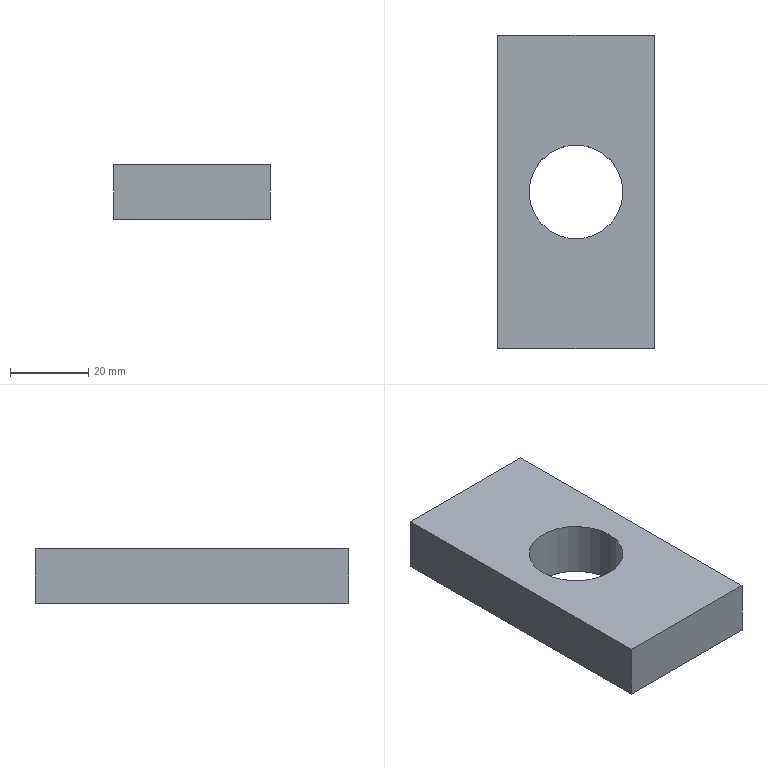Part | SolidWorks | features Extrusion 1 | 1 solid | 8 faces | box 40 x 80 x 14 mm | volume 38467 mm3 | plane 6 | cylinder 2 | commonest cylinder face diameters 24 x2
STEP:
#1=CARTESIAN_POINT('',(8.,40.,14.));
#2=VERTEX_POINT('',#1);
#3=CARTESIAN_POINT('',(32.,40.,14.));
#4=VERTEX_POINT('',#3);
#5=CARTESIAN_POINT('',(20.,40.,14.));
#6=DIRECTION('',(0.,0.,1.));
#7=DIRECTION('',(1.,0.,0.));
#8=AXIS2_PLACEMENT_3D('',#5,#6,#7);
#9=CIRCLE('',#8,12.);
#10=EDGE_CURVE('',#2,#4,#9,.T.);
#11=ORIENTED_EDGE('',*,*,#10,.T.);
#12=CARTESIAN_POINT('',(32.,40.,0.));
#13=VERTEX_POINT('',#12);
#14=CARTESIAN_POINT('',(32.,40.,14.));
#15=DIRECTION('',(0.,0.,-1.));
#16=VECTOR('',#15,1000.);
#17=LINE('',#14,#16);
#18=EDGE_CURVE('',#4,#13,#17,.T.);
#19=ORIENTED_EDGE('',*,*,#18,.T.);
#20=CARTESIAN_POINT('',(8.,40.,0.));
#21=VERTEX_POINT('',#20);
#22=CARTESIAN_POINT('',(20.,40.,0.));
#23=DIRECTION('',(0.,0.,1.));
#24=DIRECTION('',(1.,0.,0.));
#25=AXIS2_PLACEMENT_3D('',#22,#23,#24);
#26=CIRCLE('',#25,12.);
#27=EDGE_CURVE('',#21,#13,#26,.T.);
#28=ORIENTED_EDGE('',*,*,#27,.F.);
#29=CARTESIAN_POINT('',(8.,40.,14.));
#30=DIRECTION('',(0.,0.,-1.));
#31=VECTOR('',#30,1000.);
#32=LINE('',#29,#31);
#33=EDGE_CURVE('',#2,#21,#32,.T.);
#34=ORIENTED_EDGE('',*,*,#33,.F.);
#35=EDGE_LOOP('',(#11,#19,#28,#34));
#36=FACE_OUTER_BOUND('',#35,.T.);
#37=CARTESIAN_POINT('',(20.,40.,14.));
#38=DIRECTION('',(0.,0.,-1.));
#39=DIRECTION('',(-1.,0.,0.));
#40=AXIS2_PLACEMENT_3D('',#37,#38,#39);
#41=CYLINDRICAL_SURFACE('',#40,12.);
#42=ADVANCED_FACE('',(#36),#41,.F.);
#43=CARTESIAN_POINT('',(0.,80.,14.));
#44=VERTEX_POINT('',#43);
#45=CARTESIAN_POINT('',(0.,0.,14.));
#46=VERTEX_POINT('',#45);
#47=CARTESIAN_POINT('',(0.,80.,14.));
#48=DIRECTION('',(0.,-1.,0.));
#49=VECTOR('',#48,1000.);
#50=LINE('',#47,#49);
#51=EDGE_CURVE('',#44,#46,#50,.T.);
#52=ORIENTED_EDGE('',*,*,#51,.T.);
#53=CARTESIAN_POINT('',(40.,0.,14.));
#54=VERTEX_POINT('',#53);
#55=CARTESIAN_POINT('',(0.,0.,14.));
#56=DIRECTION('',(1.,0.,0.));
#57=VECTOR('',#56,1000.);
#58=LINE('',#55,#57);
#59=EDGE_CURVE('',#46,#54,#58,.T.);
#60=ORIENTED_EDGE('',*,*,#59,.T.);
#61=CARTESIAN_POINT('',(40.,80.,14.));
#62=VERTEX_POINT('',#61);
#63=CARTESIAN_POINT('',(40.,0.,14.));
#64=DIRECTION('',(0.,1.,0.));
#65=VECTOR('',#64,1000.);
#66=LINE('',#63,#65);
#67=EDGE_CURVE('',#54,#62,#66,.T.);
#68=ORIENTED_EDGE('',*,*,#67,.T.);
#69=CARTESIAN_POINT('',(40.,80.,14.));
#70=DIRECTION('',(-1.,0.,0.));
#71=VECTOR('',#70,1000.);
#72=LINE('',#69,#71);
#73=EDGE_CURVE('',#62,#44,#72,.T.);
#74=ORIENTED_EDGE('',*,*,#73,.T.);
#75=EDGE_LOOP('',(#52,#60,#68,#74));
#76=FACE_OUTER_BOUND('',#75,.T.);
#77=ORIENTED_EDGE('',*,*,#10,.F.);
#78=CARTESIAN_POINT('',(20.,40.,14.));
#79=DIRECTION('',(0.,0.,1.));
#80=DIRECTION('',(1.,0.,0.));
#81=AXIS2_PLACEMENT_3D('',#78,#79,#80);
#82=CIRCLE('',#81,12.);
#83=EDGE_CURVE('',#4,#2,#82,.T.);
#84=ORIENTED_EDGE('',*,*,#83,.F.);
#85=EDGE_LOOP('',(#77,#84));
#86=FACE_BOUND('',#85,.T.);
#87=CARTESIAN_POINT('',(0.,0.,14.));
#88=DIRECTION('',(0.,0.,1.));
#89=DIRECTION('',(1.,0.,0.));
#90=AXIS2_PLACEMENT_3D('',#87,#88,#89);
#91=PLANE('',#90);
#92=ADVANCED_FACE('',(#76,#86),#91,.T.);
#93=CARTESIAN_POINT('',(0.,80.,0.));
#94=VERTEX_POINT('',#93);
#95=CARTESIAN_POINT('',(0.,0.,0.));
#96=VERTEX_POINT('',#95);
#97=CARTESIAN_POINT('',(0.,80.,0.));
#98=DIRECTION('',(0.,-1.,0.));
#99=VECTOR('',#98,1000.);
#100=LINE('',#97,#99);
#101=EDGE_CURVE('',#94,#96,#100,.T.);
#102=ORIENTED_EDGE('',*,*,#101,.F.);
#103=CARTESIAN_POINT('',(40.,80.,0.));
#104=VERTEX_POINT('',#103);
#105=CARTESIAN_POINT('',(40.,80.,0.));
#106=DIRECTION('',(-1.,0.,0.));
#107=VECTOR('',#106,1000.);
#108=LINE('',#105,#107);
#109=EDGE_CURVE('',#104,#94,#108,.T.);
#110=ORIENTED_EDGE('',*,*,#109,.F.);
#111=CARTESIAN_POINT('',(40.,0.,0.));
#112=VERTEX_POINT('',#111);
#113=CARTESIAN_POINT('',(40.,0.,0.));
#114=DIRECTION('',(0.,1.,0.));
#115=VECTOR('',#114,1000.);
#116=LINE('',#113,#115);
#117=EDGE_CURVE('',#112,#104,#116,.T.);
#118=ORIENTED_EDGE('',*,*,#117,.F.);
#119=CARTESIAN_POINT('',(0.,0.,0.));
#120=DIRECTION('',(1.,0.,0.));
#121=VECTOR('',#120,1000.);
#122=LINE('',#119,#121);
#123=EDGE_CURVE('',#96,#112,#122,.T.);
#124=ORIENTED_EDGE('',*,*,#123,.F.);
#125=EDGE_LOOP('',(#102,#110,#118,#124));
#126=FACE_OUTER_BOUND('',#125,.T.);
#127=ORIENTED_EDGE('',*,*,#27,.T.);
#128=CARTESIAN_POINT('',(20.,40.,0.));
#129=DIRECTION('',(0.,0.,1.));
#130=DIRECTION('',(1.,0.,0.));
#131=AXIS2_PLACEMENT_3D('',#128,#129,#130);
#132=CIRCLE('',#131,12.);
#133=EDGE_CURVE('',#13,#21,#132,.T.);
#134=ORIENTED_EDGE('',*,*,#133,.T.);
#135=EDGE_LOOP('',(#127,#134));
#136=FACE_BOUND('',#135,.T.);
#137=CARTESIAN_POINT('',(0.,0.,0.));
#138=DIRECTION('',(0.,0.,1.));
#139=DIRECTION('',(1.,0.,0.));
#140=AXIS2_PLACEMENT_3D('',#137,#138,#139);
#141=PLANE('',#140);
#142=ADVANCED_FACE('',(#126,#136),#141,.F.);
#143=ORIENTED_EDGE('',*,*,#101,.T.);
#144=CARTESIAN_POINT('',(0.,0.,14.));
#145=DIRECTION('',(0.,0.,-1.));
#146=VECTOR('',#145,1000.);
#147=LINE('',#144,#146);
#148=EDGE_CURVE('',#46,#96,#147,.T.);
#149=ORIENTED_EDGE('',*,*,#148,.F.);
#150=ORIENTED_EDGE('',*,*,#51,.F.);
#151=CARTESIAN_POINT('',(0.,80.,14.));
#152=DIRECTION('',(0.,0.,-1.));
#153=VECTOR('',#152,1000.);
#154=LINE('',#151,#153);
#155=EDGE_CURVE('',#44,#94,#154,.T.);
#156=ORIENTED_EDGE('',*,*,#155,.T.);
#157=EDGE_LOOP('',(#143,#149,#150,#156));
#158=FACE_OUTER_BOUND('',#157,.T.);
#159=CARTESIAN_POINT('',(0.,80.,14.));
#160=DIRECTION('',(1.,0.,0.));
#161=DIRECTION('',(0.,1.,0.));
#162=AXIS2_PLACEMENT_3D('',#159,#160,#161);
#163=PLANE('',#162);
#164=ADVANCED_FACE('',(#158),#163,.F.);
#165=ORIENTED_EDGE('',*,*,#123,.T.);
#166=CARTESIAN_POINT('',(40.,0.,14.));
#167=DIRECTION('',(0.,0.,-1.));
#168=VECTOR('',#167,1000.);
#169=LINE('',#166,#168);
#170=EDGE_CURVE('',#54,#112,#169,.T.);
#171=ORIENTED_EDGE('',*,*,#170,.F.);
#172=ORIENTED_EDGE('',*,*,#59,.F.);
#173=ORIENTED_EDGE('',*,*,#148,.T.);
#174=EDGE_LOOP('',(#165,#171,#172,#173));
#175=FACE_OUTER_BOUND('',#174,.T.);
#176=CARTESIAN_POINT('',(0.,0.,14.));
#177=DIRECTION('',(0.,1.,0.));
#178=DIRECTION('',(0.,0.,1.));
#179=AXIS2_PLACEMENT_3D('',#176,#177,#178);
#180=PLANE('',#179);
#181=ADVANCED_FACE('',(#175),#180,.F.);
#182=ORIENTED_EDGE('',*,*,#117,.T.);
#183=CARTESIAN_POINT('',(40.,80.,14.));
#184=DIRECTION('',(0.,0.,-1.));
#185=VECTOR('',#184,1000.);
#186=LINE('',#183,#185);
#187=EDGE_CURVE('',#62,#104,#186,.T.);
#188=ORIENTED_EDGE('',*,*,#187,.F.);
#189=ORIENTED_EDGE('',*,*,#67,.F.);
#190=ORIENTED_EDGE('',*,*,#170,.T.);
#191=EDGE_LOOP('',(#182,#188,#189,#190));
#192=FACE_OUTER_BOUND('',#191,.T.);
#193=CARTESIAN_POINT('',(40.,0.,14.));
#194=DIRECTION('',(-1.,0.,0.));
#195=DIRECTION('',(0.,0.,1.));
#196=AXIS2_PLACEMENT_3D('',#193,#194,#195);
#197=PLANE('',#196);
#198=ADVANCED_FACE('',(#192),#197,.F.);
#199=ORIENTED_EDGE('',*,*,#109,.T.);
#200=ORIENTED_EDGE('',*,*,#155,.F.);
#201=ORIENTED_EDGE('',*,*,#73,.F.);
#202=ORIENTED_EDGE('',*,*,#187,.T.);
#203=EDGE_LOOP('',(#199,#200,#201,#202));
#204=FACE_OUTER_BOUND('',#203,.T.);
#205=CARTESIAN_POINT('',(40.,80.,14.));
#206=DIRECTION('',(0.,-1.,0.));
#207=DIRECTION('',(1.,0.,0.));
#208=AXIS2_PLACEMENT_3D('',#205,#206,#207);
#209=PLANE('',#208);
#210=ADVANCED_FACE('',(#204),#209,.F.);
#211=ORIENTED_EDGE('',*,*,#18,.F.);
#212=ORIENTED_EDGE('',*,*,#83,.T.);
#213=ORIENTED_EDGE('',*,*,#33,.T.);
#214=ORIENTED_EDGE('',*,*,#133,.F.);
#215=EDGE_LOOP('',(#211,#212,#213,#214));
#216=FACE_OUTER_BOUND('',#215,.T.);
#217=CARTESIAN_POINT('',(20.,40.,14.));
#218=DIRECTION('',(0.,0.,-1.));
#219=DIRECTION('',(-1.,0.,0.));
#220=AXIS2_PLACEMENT_3D('',#217,#218,#219);
#221=CYLINDRICAL_SURFACE('',#220,12.);
#222=ADVANCED_FACE('',(#216),#221,.F.);
#223=CLOSED_SHELL('',(#42,#92,#142,#164,#181,#198,#210,#222));
#224=MANIFOLD_SOLID_BREP('',#223);
#225=CARTESIAN_POINT('',(0.,0.,0.));
#226=DIRECTION('',(0.,0.,1.));
#227=DIRECTION('',(1.,0.,0.));
#228=AXIS2_PLACEMENT_3D('',#225,#226,#227);
#229=(LENGTH_UNIT()NAMED_UNIT(*)SI_UNIT(.MILLI.,.METRE.));
#230=UNCERTAINTY_MEASURE_WITH_UNIT(LENGTH_MEASURE(0.00001),#229,'','');
#231=(NAMED_UNIT(*)PLANE_ANGLE_UNIT()SI_UNIT($,.RADIAN.));
#232=(NAMED_UNIT(*)SI_UNIT($,.STERADIAN.)SOLID_ANGLE_UNIT());
#233=(GEOMETRIC_REPRESENTATION_CONTEXT(3)GLOBAL_UNCERTAINTY_ASSIGNED_CONTEXT((#230))GLOBAL_UNIT_ASSIGNED_CONTEXT((#229,#231,#232))REPRESENTATION_CONTEXT('',''));
#234=ADVANCED_BREP_SHAPE_REPRESENTATION('',(#224,#228),#233);